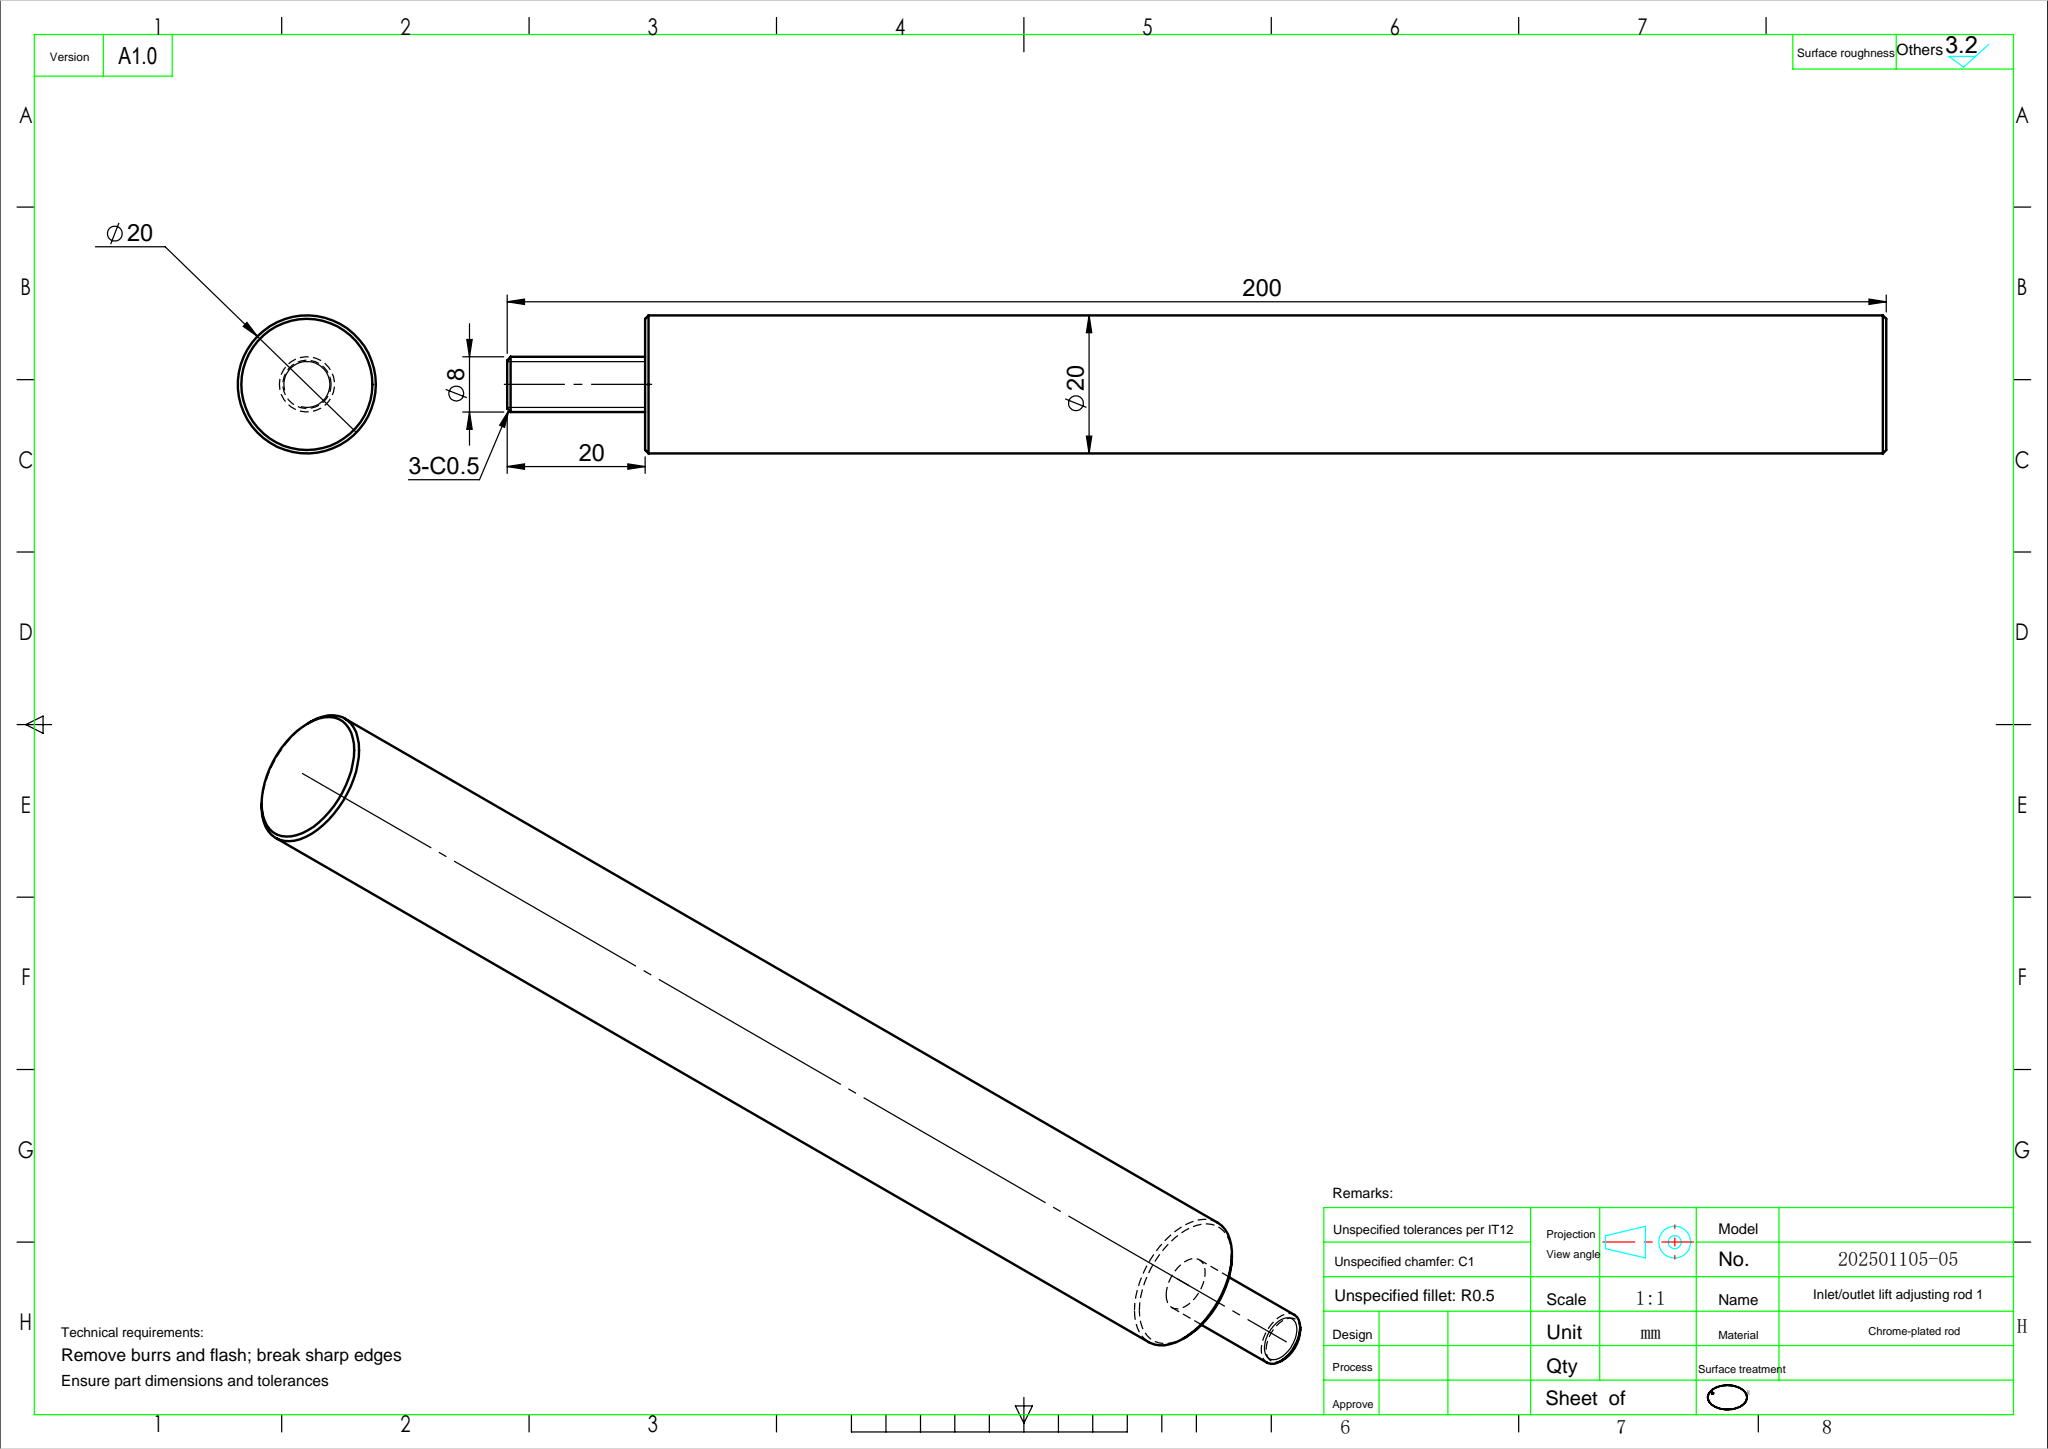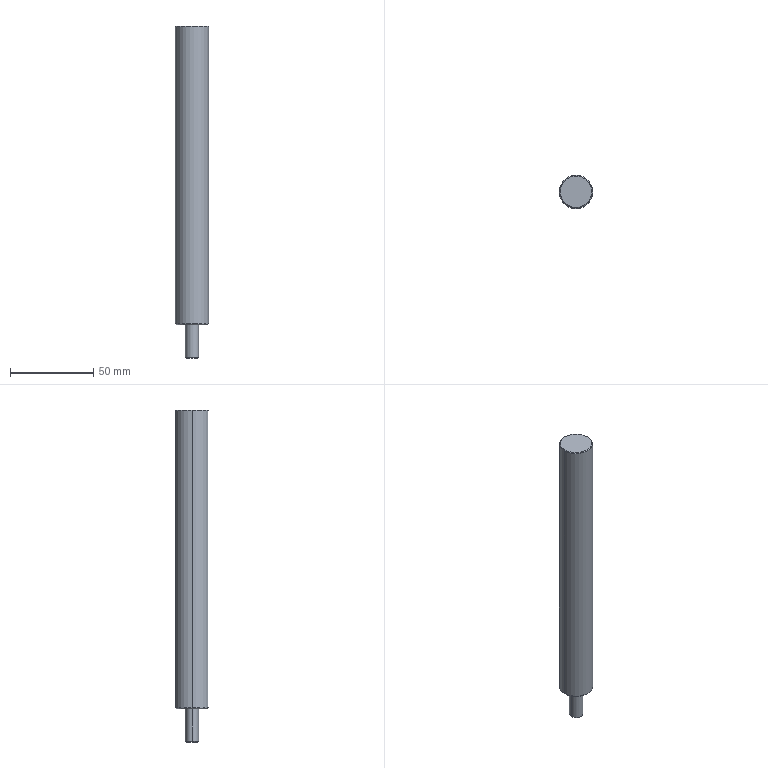Part | SolidWorks | features Chamfer 1, Extrusion 1, ICE 1 | 1 solid | 13 faces | box 20 x 20 x 200 mm | volume 57536 mm3 | cone 6 | cylinder 4 | plane 3 | commonest cylinder face diameters 8 x2 20 x2
STEP:
#1=CARTESIAN_POINT('',(9.5,0.,200.));
#2=VERTEX_POINT('',#1);
#3=CARTESIAN_POINT('',(-9.5,0.,200.));
#4=VERTEX_POINT('',#3);
#5=CARTESIAN_POINT('',(0.,0.,200.));
#6=DIRECTION('',(0.,0.,1.));
#7=DIRECTION('',(1.,0.,0.));
#8=AXIS2_PLACEMENT_3D('',#5,#6,#7);
#9=CIRCLE('',#8,9.5);
#10=EDGE_CURVE('',#2,#4,#9,.T.);
#11=ORIENTED_EDGE('',*,*,#10,.F.);
#12=CARTESIAN_POINT('',(10.,0.,199.5));
#13=VERTEX_POINT('',#12);
#14=CARTESIAN_POINT('',(9.5,0.,200.));
#15=DIRECTION('',(0.7071,0.,-0.7071));
#16=VECTOR('',#15,1000.);
#17=LINE('',#14,#16);
#18=EDGE_CURVE('',#2,#13,#17,.T.);
#19=ORIENTED_EDGE('',*,*,#18,.T.);
#20=CARTESIAN_POINT('',(-10.,0.,199.5));
#21=VERTEX_POINT('',#20);
#22=CARTESIAN_POINT('',(0.,0.,199.5));
#23=DIRECTION('',(0.,0.,-1.));
#24=DIRECTION('',(1.,0.,0.));
#25=AXIS2_PLACEMENT_3D('',#22,#23,#24);
#26=CIRCLE('',#25,10.);
#27=EDGE_CURVE('',#21,#13,#26,.T.);
#28=ORIENTED_EDGE('',*,*,#27,.F.);
#29=CARTESIAN_POINT('',(-9.5,0.,200.));
#30=DIRECTION('',(-0.7071,0.,-0.7071));
#31=VECTOR('',#30,1000.);
#32=LINE('',#29,#31);
#33=EDGE_CURVE('',#4,#21,#32,.T.);
#34=ORIENTED_EDGE('',*,*,#33,.F.);
#35=EDGE_LOOP('',(#11,#19,#28,#34));
#36=FACE_OUTER_BOUND('',#35,.T.);
#37=CARTESIAN_POINT('',(0.,0.,200.));
#38=DIRECTION('',(0.,0.,-1.));
#39=DIRECTION('',(-1.,0.,0.));
#40=AXIS2_PLACEMENT_3D('',#37,#38,#39);
#41=CONICAL_SURFACE('',#40,9.5,0.7854);
#42=ADVANCED_FACE('',(#36),#41,.T.);
#43=CARTESIAN_POINT('',(-9.5,0.,20.));
#44=VERTEX_POINT('',#43);
#45=CARTESIAN_POINT('',(9.5,0.,20.));
#46=VERTEX_POINT('',#45);
#47=CARTESIAN_POINT('',(0.,0.,20.));
#48=DIRECTION('',(0.,0.,-1.));
#49=DIRECTION('',(-1.,0.,0.));
#50=AXIS2_PLACEMENT_3D('',#47,#48,#49);
#51=CIRCLE('',#50,9.5);
#52=EDGE_CURVE('',#44,#46,#51,.T.);
#53=ORIENTED_EDGE('',*,*,#52,.F.);
#54=CARTESIAN_POINT('',(-10.,0.,20.5));
#55=VERTEX_POINT('',#54);
#56=CARTESIAN_POINT('',(-9.5,0.,20.));
#57=DIRECTION('',(-0.7071,0.,0.7071));
#58=VECTOR('',#57,1000.);
#59=LINE('',#56,#58);
#60=EDGE_CURVE('',#44,#55,#59,.T.);
#61=ORIENTED_EDGE('',*,*,#60,.T.);
#62=CARTESIAN_POINT('',(10.,0.,20.5));
#63=VERTEX_POINT('',#62);
#64=CARTESIAN_POINT('',(0.,0.,20.5));
#65=DIRECTION('',(0.,0.,1.));
#66=DIRECTION('',(-1.,0.,0.));
#67=AXIS2_PLACEMENT_3D('',#64,#65,#66);
#68=CIRCLE('',#67,10.);
#69=EDGE_CURVE('',#63,#55,#68,.T.);
#70=ORIENTED_EDGE('',*,*,#69,.F.);
#71=CARTESIAN_POINT('',(9.5,0.,20.));
#72=DIRECTION('',(0.7071,0.,0.7071));
#73=VECTOR('',#72,1000.);
#74=LINE('',#71,#73);
#75=EDGE_CURVE('',#46,#63,#74,.T.);
#76=ORIENTED_EDGE('',*,*,#75,.F.);
#77=EDGE_LOOP('',(#53,#61,#70,#76));
#78=FACE_OUTER_BOUND('',#77,.T.);
#79=CARTESIAN_POINT('',(0.,0.,20.));
#80=DIRECTION('',(0.,0.,1.));
#81=DIRECTION('',(1.,0.,0.));
#82=AXIS2_PLACEMENT_3D('',#79,#80,#81);
#83=CONICAL_SURFACE('',#82,9.5,0.7854);
#84=ADVANCED_FACE('',(#78),#83,.T.);
#85=CARTESIAN_POINT('',(-3.5,0.,0.));
#86=VERTEX_POINT('',#85);
#87=CARTESIAN_POINT('',(3.5,0.,0.));
#88=VERTEX_POINT('',#87);
#89=CARTESIAN_POINT('',(0.,0.,0.));
#90=DIRECTION('',(0.,0.,-1.));
#91=DIRECTION('',(1.,0.,0.));
#92=AXIS2_PLACEMENT_3D('',#89,#90,#91);
#93=CIRCLE('',#92,3.5);
#94=EDGE_CURVE('',#86,#88,#93,.T.);
#95=ORIENTED_EDGE('',*,*,#94,.F.);
#96=CARTESIAN_POINT('',(-4.,0.,0.5));
#97=VERTEX_POINT('',#96);
#98=CARTESIAN_POINT('',(-3.5,0.,0.));
#99=DIRECTION('',(-0.7071,0.,0.7071));
#100=VECTOR('',#99,1000.);
#101=LINE('',#98,#100);
#102=EDGE_CURVE('',#86,#97,#101,.T.);
#103=ORIENTED_EDGE('',*,*,#102,.T.);
#104=CARTESIAN_POINT('',(4.,0.,0.5));
#105=VERTEX_POINT('',#104);
#106=CARTESIAN_POINT('',(0.,0.,0.5));
#107=DIRECTION('',(0.,0.,1.));
#108=DIRECTION('',(1.,0.,0.));
#109=AXIS2_PLACEMENT_3D('',#106,#107,#108);
#110=CIRCLE('',#109,4.);
#111=EDGE_CURVE('',#105,#97,#110,.T.);
#112=ORIENTED_EDGE('',*,*,#111,.F.);
#113=CARTESIAN_POINT('',(3.5,0.,0.));
#114=DIRECTION('',(0.7071,0.,0.7071));
#115=VECTOR('',#114,1000.);
#116=LINE('',#113,#115);
#117=EDGE_CURVE('',#88,#105,#116,.T.);
#118=ORIENTED_EDGE('',*,*,#117,.F.);
#119=EDGE_LOOP('',(#95,#103,#112,#118));
#120=FACE_OUTER_BOUND('',#119,.T.);
#121=CARTESIAN_POINT('',(0.,0.,0.));
#122=DIRECTION('',(0.,0.,1.));
#123=DIRECTION('',(1.,0.,0.));
#124=AXIS2_PLACEMENT_3D('',#121,#122,#123);
#125=CONICAL_SURFACE('',#124,3.5,0.7854);
#126=ADVANCED_FACE('',(#120),#125,.T.);
#127=CARTESIAN_POINT('',(-4.,0.,20.));
#128=VERTEX_POINT('',#127);
#129=CARTESIAN_POINT('',(4.,0.,20.));
#130=VERTEX_POINT('',#129);
#131=CARTESIAN_POINT('',(0.,0.,20.));
#132=DIRECTION('',(0.,0.,-1.));
#133=DIRECTION('',(-1.,0.,0.));
#134=AXIS2_PLACEMENT_3D('',#131,#132,#133);
#135=CIRCLE('',#134,4.);
#136=EDGE_CURVE('',#128,#130,#135,.T.);
#137=ORIENTED_EDGE('',*,*,#136,.T.);
#138=CARTESIAN_POINT('',(4.,0.,20.));
#139=DIRECTION('',(0.,0.,-1.));
#140=VECTOR('',#139,1000.);
#141=LINE('',#138,#140);
#142=EDGE_CURVE('',#130,#105,#141,.T.);
#143=ORIENTED_EDGE('',*,*,#142,.T.);
#144=ORIENTED_EDGE('',*,*,#111,.T.);
#145=CARTESIAN_POINT('',(-4.,0.,20.));
#146=DIRECTION('',(0.,0.,-1.));
#147=VECTOR('',#146,1000.);
#148=LINE('',#145,#147);
#149=EDGE_CURVE('',#128,#97,#148,.T.);
#150=ORIENTED_EDGE('',*,*,#149,.F.);
#151=EDGE_LOOP('',(#137,#143,#144,#150));
#152=FACE_OUTER_BOUND('',#151,.T.);
#153=CARTESIAN_POINT('',(0.,0.,20.));
#154=DIRECTION('',(0.,0.,-1.));
#155=DIRECTION('',(-1.,0.,0.));
#156=AXIS2_PLACEMENT_3D('',#153,#154,#155);
#157=CYLINDRICAL_SURFACE('',#156,4.);
#158=ADVANCED_FACE('',(#152),#157,.T.);
#159=ORIENTED_EDGE('',*,*,#27,.T.);
#160=CARTESIAN_POINT('',(10.,0.,200.));
#161=DIRECTION('',(0.,0.,-1.));
#162=VECTOR('',#161,1000.);
#163=LINE('',#160,#162);
#164=EDGE_CURVE('',#13,#63,#163,.T.);
#165=ORIENTED_EDGE('',*,*,#164,.T.);
#166=ORIENTED_EDGE('',*,*,#69,.T.);
#167=CARTESIAN_POINT('',(-10.,0.,200.));
#168=DIRECTION('',(0.,0.,-1.));
#169=VECTOR('',#168,1000.);
#170=LINE('',#167,#169);
#171=EDGE_CURVE('',#21,#55,#170,.T.);
#172=ORIENTED_EDGE('',*,*,#171,.F.);
#173=EDGE_LOOP('',(#159,#165,#166,#172));
#174=FACE_OUTER_BOUND('',#173,.T.);
#175=CARTESIAN_POINT('',(0.,0.,200.));
#176=DIRECTION('',(0.,0.,-1.));
#177=DIRECTION('',(-1.,0.,0.));
#178=AXIS2_PLACEMENT_3D('',#175,#176,#177);
#179=CYLINDRICAL_SURFACE('',#178,10.);
#180=ADVANCED_FACE('',(#174),#179,.T.);
#181=ORIENTED_EDGE('',*,*,#164,.F.);
#182=CARTESIAN_POINT('',(0.,0.,199.5));
#183=DIRECTION('',(0.,0.,-1.));
#184=DIRECTION('',(1.,0.,0.));
#185=AXIS2_PLACEMENT_3D('',#182,#183,#184);
#186=CIRCLE('',#185,10.);
#187=EDGE_CURVE('',#13,#21,#186,.T.);
#188=ORIENTED_EDGE('',*,*,#187,.T.);
#189=ORIENTED_EDGE('',*,*,#171,.T.);
#190=CARTESIAN_POINT('',(0.,0.,20.5));
#191=DIRECTION('',(0.,0.,1.));
#192=DIRECTION('',(-1.,0.,0.));
#193=AXIS2_PLACEMENT_3D('',#190,#191,#192);
#194=CIRCLE('',#193,10.);
#195=EDGE_CURVE('',#55,#63,#194,.T.);
#196=ORIENTED_EDGE('',*,*,#195,.T.);
#197=EDGE_LOOP('',(#181,#188,#189,#196));
#198=FACE_OUTER_BOUND('',#197,.T.);
#199=CARTESIAN_POINT('',(0.,0.,200.));
#200=DIRECTION('',(0.,0.,-1.));
#201=DIRECTION('',(-1.,0.,0.));
#202=AXIS2_PLACEMENT_3D('',#199,#200,#201);
#203=CYLINDRICAL_SURFACE('',#202,10.);
#204=ADVANCED_FACE('',(#198),#203,.T.);
#205=CARTESIAN_POINT('',(0.,0.,200.));
#206=DIRECTION('',(0.,0.,1.));
#207=DIRECTION('',(1.,0.,0.));
#208=AXIS2_PLACEMENT_3D('',#205,#206,#207);
#209=CIRCLE('',#208,9.5);
#210=EDGE_CURVE('',#4,#2,#209,.T.);
#211=ORIENTED_EDGE('',*,*,#210,.T.);
#212=ORIENTED_EDGE('',*,*,#10,.T.);
#213=EDGE_LOOP('',(#211,#212));
#214=FACE_OUTER_BOUND('',#213,.T.);
#215=CARTESIAN_POINT('',(0.,0.,200.));
#216=DIRECTION('',(0.,0.,1.));
#217=DIRECTION('',(1.,0.,0.));
#218=AXIS2_PLACEMENT_3D('',#215,#216,#217);
#219=PLANE('',#218);
#220=ADVANCED_FACE('',(#214),#219,.T.);
#221=CARTESIAN_POINT('',(0.,0.,20.));
#222=DIRECTION('',(0.,0.,-1.));
#223=DIRECTION('',(-1.,0.,0.));
#224=AXIS2_PLACEMENT_3D('',#221,#222,#223);
#225=CIRCLE('',#224,9.5);
#226=EDGE_CURVE('',#46,#44,#225,.T.);
#227=ORIENTED_EDGE('',*,*,#226,.T.);
#228=ORIENTED_EDGE('',*,*,#52,.T.);
#229=EDGE_LOOP('',(#227,#228));
#230=FACE_OUTER_BOUND('',#229,.T.);
#231=ORIENTED_EDGE('',*,*,#136,.F.);
#232=CARTESIAN_POINT('',(0.,0.,20.));
#233=DIRECTION('',(0.,0.,-1.));
#234=DIRECTION('',(-1.,0.,0.));
#235=AXIS2_PLACEMENT_3D('',#232,#233,#234);
#236=CIRCLE('',#235,4.);
#237=EDGE_CURVE('',#130,#128,#236,.T.);
#238=ORIENTED_EDGE('',*,*,#237,.F.);
#239=EDGE_LOOP('',(#231,#238));
#240=FACE_BOUND('',#239,.T.);
#241=CARTESIAN_POINT('',(0.,0.,20.));
#242=DIRECTION('',(0.,0.,-1.));
#243=DIRECTION('',(-1.,0.,0.));
#244=AXIS2_PLACEMENT_3D('',#241,#242,#243);
#245=PLANE('',#244);
#246=ADVANCED_FACE('',(#230,#240),#245,.T.);
#247=ORIENTED_EDGE('',*,*,#142,.F.);
#248=ORIENTED_EDGE('',*,*,#237,.T.);
#249=ORIENTED_EDGE('',*,*,#149,.T.);
#250=CARTESIAN_POINT('',(0.,0.,0.5));
#251=DIRECTION('',(0.,0.,1.));
#252=DIRECTION('',(1.,0.,0.));
#253=AXIS2_PLACEMENT_3D('',#250,#251,#252);
#254=CIRCLE('',#253,4.);
#255=EDGE_CURVE('',#97,#105,#254,.T.);
#256=ORIENTED_EDGE('',*,*,#255,.T.);
#257=EDGE_LOOP('',(#247,#248,#249,#256));
#258=FACE_OUTER_BOUND('',#257,.T.);
#259=CARTESIAN_POINT('',(0.,0.,20.));
#260=DIRECTION('',(0.,0.,-1.));
#261=DIRECTION('',(-1.,0.,0.));
#262=AXIS2_PLACEMENT_3D('',#259,#260,#261);
#263=CYLINDRICAL_SURFACE('',#262,4.);
#264=ADVANCED_FACE('',(#258),#263,.T.);
#265=CARTESIAN_POINT('',(0.,0.,0.));
#266=DIRECTION('',(0.,0.,-1.));
#267=DIRECTION('',(1.,0.,0.));
#268=AXIS2_PLACEMENT_3D('',#265,#266,#267);
#269=CIRCLE('',#268,3.5);
#270=EDGE_CURVE('',#88,#86,#269,.T.);
#271=ORIENTED_EDGE('',*,*,#270,.T.);
#272=ORIENTED_EDGE('',*,*,#94,.T.);
#273=EDGE_LOOP('',(#271,#272));
#274=FACE_OUTER_BOUND('',#273,.T.);
#275=CARTESIAN_POINT('',(0.,0.,0.));
#276=DIRECTION('',(0.,0.,1.));
#277=DIRECTION('',(1.,0.,0.));
#278=AXIS2_PLACEMENT_3D('',#275,#276,#277);
#279=PLANE('',#278);
#280=ADVANCED_FACE('',(#274),#279,.F.);
#281=ORIENTED_EDGE('',*,*,#102,.F.);
#282=ORIENTED_EDGE('',*,*,#270,.F.);
#283=ORIENTED_EDGE('',*,*,#117,.T.);
#284=ORIENTED_EDGE('',*,*,#255,.F.);
#285=EDGE_LOOP('',(#281,#282,#283,#284));
#286=FACE_OUTER_BOUND('',#285,.T.);
#287=CARTESIAN_POINT('',(0.,0.,0.));
#288=DIRECTION('',(0.,0.,1.));
#289=DIRECTION('',(1.,0.,0.));
#290=AXIS2_PLACEMENT_3D('',#287,#288,#289);
#291=CONICAL_SURFACE('',#290,3.5,0.7854);
#292=ADVANCED_FACE('',(#286),#291,.T.);
#293=ORIENTED_EDGE('',*,*,#60,.F.);
#294=ORIENTED_EDGE('',*,*,#226,.F.);
#295=ORIENTED_EDGE('',*,*,#75,.T.);
#296=ORIENTED_EDGE('',*,*,#195,.F.);
#297=EDGE_LOOP('',(#293,#294,#295,#296));
#298=FACE_OUTER_BOUND('',#297,.T.);
#299=CARTESIAN_POINT('',(0.,0.,20.));
#300=DIRECTION('',(0.,0.,1.));
#301=DIRECTION('',(1.,0.,0.));
#302=AXIS2_PLACEMENT_3D('',#299,#300,#301);
#303=CONICAL_SURFACE('',#302,9.5,0.7854);
#304=ADVANCED_FACE('',(#298),#303,.T.);
#305=ORIENTED_EDGE('',*,*,#18,.F.);
#306=ORIENTED_EDGE('',*,*,#210,.F.);
#307=ORIENTED_EDGE('',*,*,#33,.T.);
#308=ORIENTED_EDGE('',*,*,#187,.F.);
#309=EDGE_LOOP('',(#305,#306,#307,#308));
#310=FACE_OUTER_BOUND('',#309,.T.);
#311=CARTESIAN_POINT('',(0.,0.,200.));
#312=DIRECTION('',(0.,0.,-1.));
#313=DIRECTION('',(-1.,0.,0.));
#314=AXIS2_PLACEMENT_3D('',#311,#312,#313);
#315=CONICAL_SURFACE('',#314,9.5,0.7854);
#316=ADVANCED_FACE('',(#310),#315,.T.);
#317=CLOSED_SHELL('',(#42,#84,#126,#158,#180,#204,#220,#246,#264,#280,#292,#304,#316));
#318=MANIFOLD_SOLID_BREP('',#317);
#319=CARTESIAN_POINT('',(0.,0.,0.));
#320=DIRECTION('',(0.,0.,1.));
#321=DIRECTION('',(1.,0.,0.));
#322=AXIS2_PLACEMENT_3D('',#319,#320,#321);
#323=(LENGTH_UNIT()NAMED_UNIT(*)SI_UNIT(.MILLI.,.METRE.));
#324=UNCERTAINTY_MEASURE_WITH_UNIT(LENGTH_MEASURE(0.00001),#323,'','');
#325=(NAMED_UNIT(*)PLANE_ANGLE_UNIT()SI_UNIT($,.RADIAN.));
#326=(NAMED_UNIT(*)SI_UNIT($,.STERADIAN.)SOLID_ANGLE_UNIT());
#327=(GEOMETRIC_REPRESENTATION_CONTEXT(3)GLOBAL_UNCERTAINTY_ASSIGNED_CONTEXT((#324))GLOBAL_UNIT_ASSIGNED_CONTEXT((#323,#325,#326))REPRESENTATION_CONTEXT('',''));
#328=ADVANCED_BREP_SHAPE_REPRESENTATION('',(#318,#322),#327);